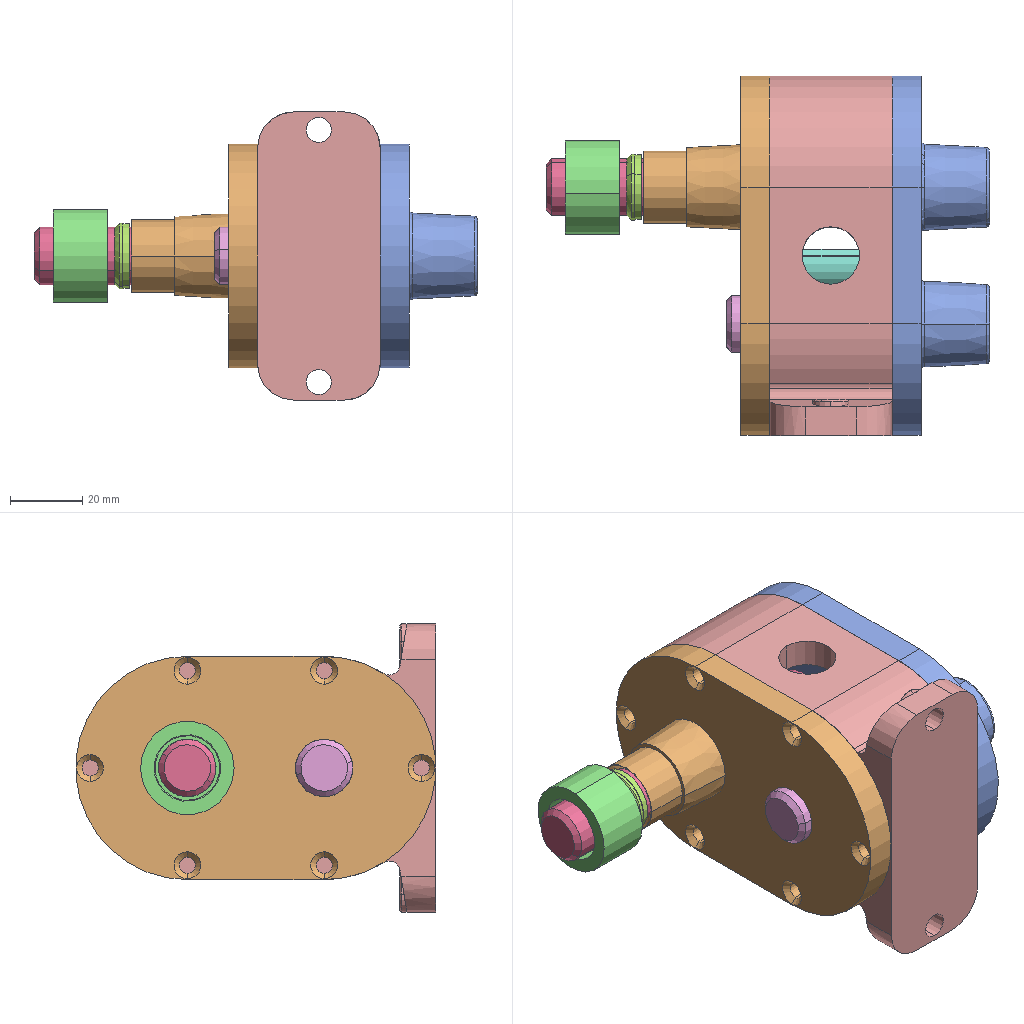Assembly | SolidWorks | 9 different items | 9 placed | box 123 x 100 x 80 mm
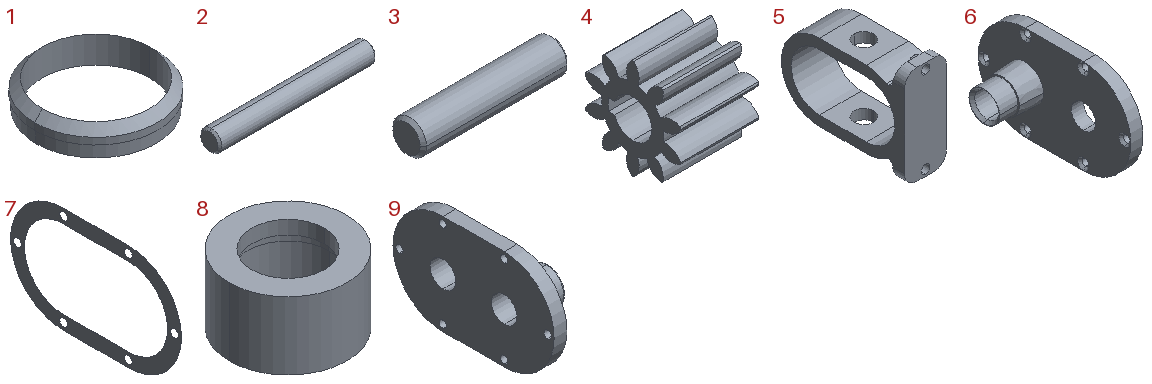Parts list (item | quantity | size | volume | features):
1 | x1 | 18.4 x 18.4 x 4 mm | 198.976 mm3 | features Revolution 1
2 | x1 | - | - | features Chamfer 1, ICE 1, RefSurface 1, Revolution 1
3 | x1 | 70 x 16 x 16 mm | 13968 mm3 | features Revolution 1
4 | x1 | 33 x 40.213 x 42 mm | 22176 mm3 | features Extrusion 1
5 | x1 | 34 x 100 x 80 mm | 78482 mm3 | features ICE 4, HoleWzd 3, Fillet 2, BaseBody 1
6 | x1 | 35 x 100 x 62 mm | 43276 mm3 | features HoleWzd 3, Chamfer 1, Extrusion 1, Revolution 1
7 | x1 | 0.05 x 100 x 62 mm | 93.487 mm3 | features Extrusion 1
8 | x1 | 26 x 26 x 15 mm | 4163 mm3 | features Revolution 1
9 | x1 | 27 x 100 x 62 mm | 48310 mm3 | features HoleWzd 2, Revolution 2, Chamfer 1, Extrusion 1, Fillet 1
Mates (type | each side: item.copy, entity, surface, feature):
Coincident | 5.1 face plane Boss-Extrude1 | 6.1 face plane Boss-Extrude1
Concentric | 5.1 face cylinder Input3 | 6.1 face cylinder Boss-Extrude1
Coincident | 5.1 face plane Boss-Extrude3 | 7.1 face plane Boss-Extrude1
Coincident | 9.1 face plane Boss-Extrude1 | 7.1 face plane Boss-Extrude1
Concentric | 5.1 face cylinder Input3 | 9.1 face cylinder Boss-Extrude1
Concentric | 9.1 face cylinder Ø4.5 (4.5) Diameter Hole1 | 7.1 face cylinder Boss-Extrude1 | 2 times
Concentric | 5.1 face cylinder Cut-Extrude1 | 4.1 face cylinder Boss-Extrude1
Coincident | 4.1 face plane Boss-Extrude1 | 6.1 face plane Boss-Extrude1
Concentric | 1.1 face cylinder Revolve1 | 6.1 face cylinder Revolve1
Concentric | 2.1 face cylinder Revolve1 | 6.1 face cylinder Ø16.0 (16) Diameter Hole2
Coincident | 9.1 face plane Ø16.0 (16) Diameter Hole1 | 2.1 face plane Revolve1
Concentric | 3.1 face cylinder Revolve1 | 4.1 face cylinder Boss-Extrude1
Coincident | 9.1 face plane Ø16.0 (16) Diameter Hole1 | 3.1 face plane Revolve1
Concentric | 2.1 face cylinder Revolve1 | 8.1 face cylinder Revolve1